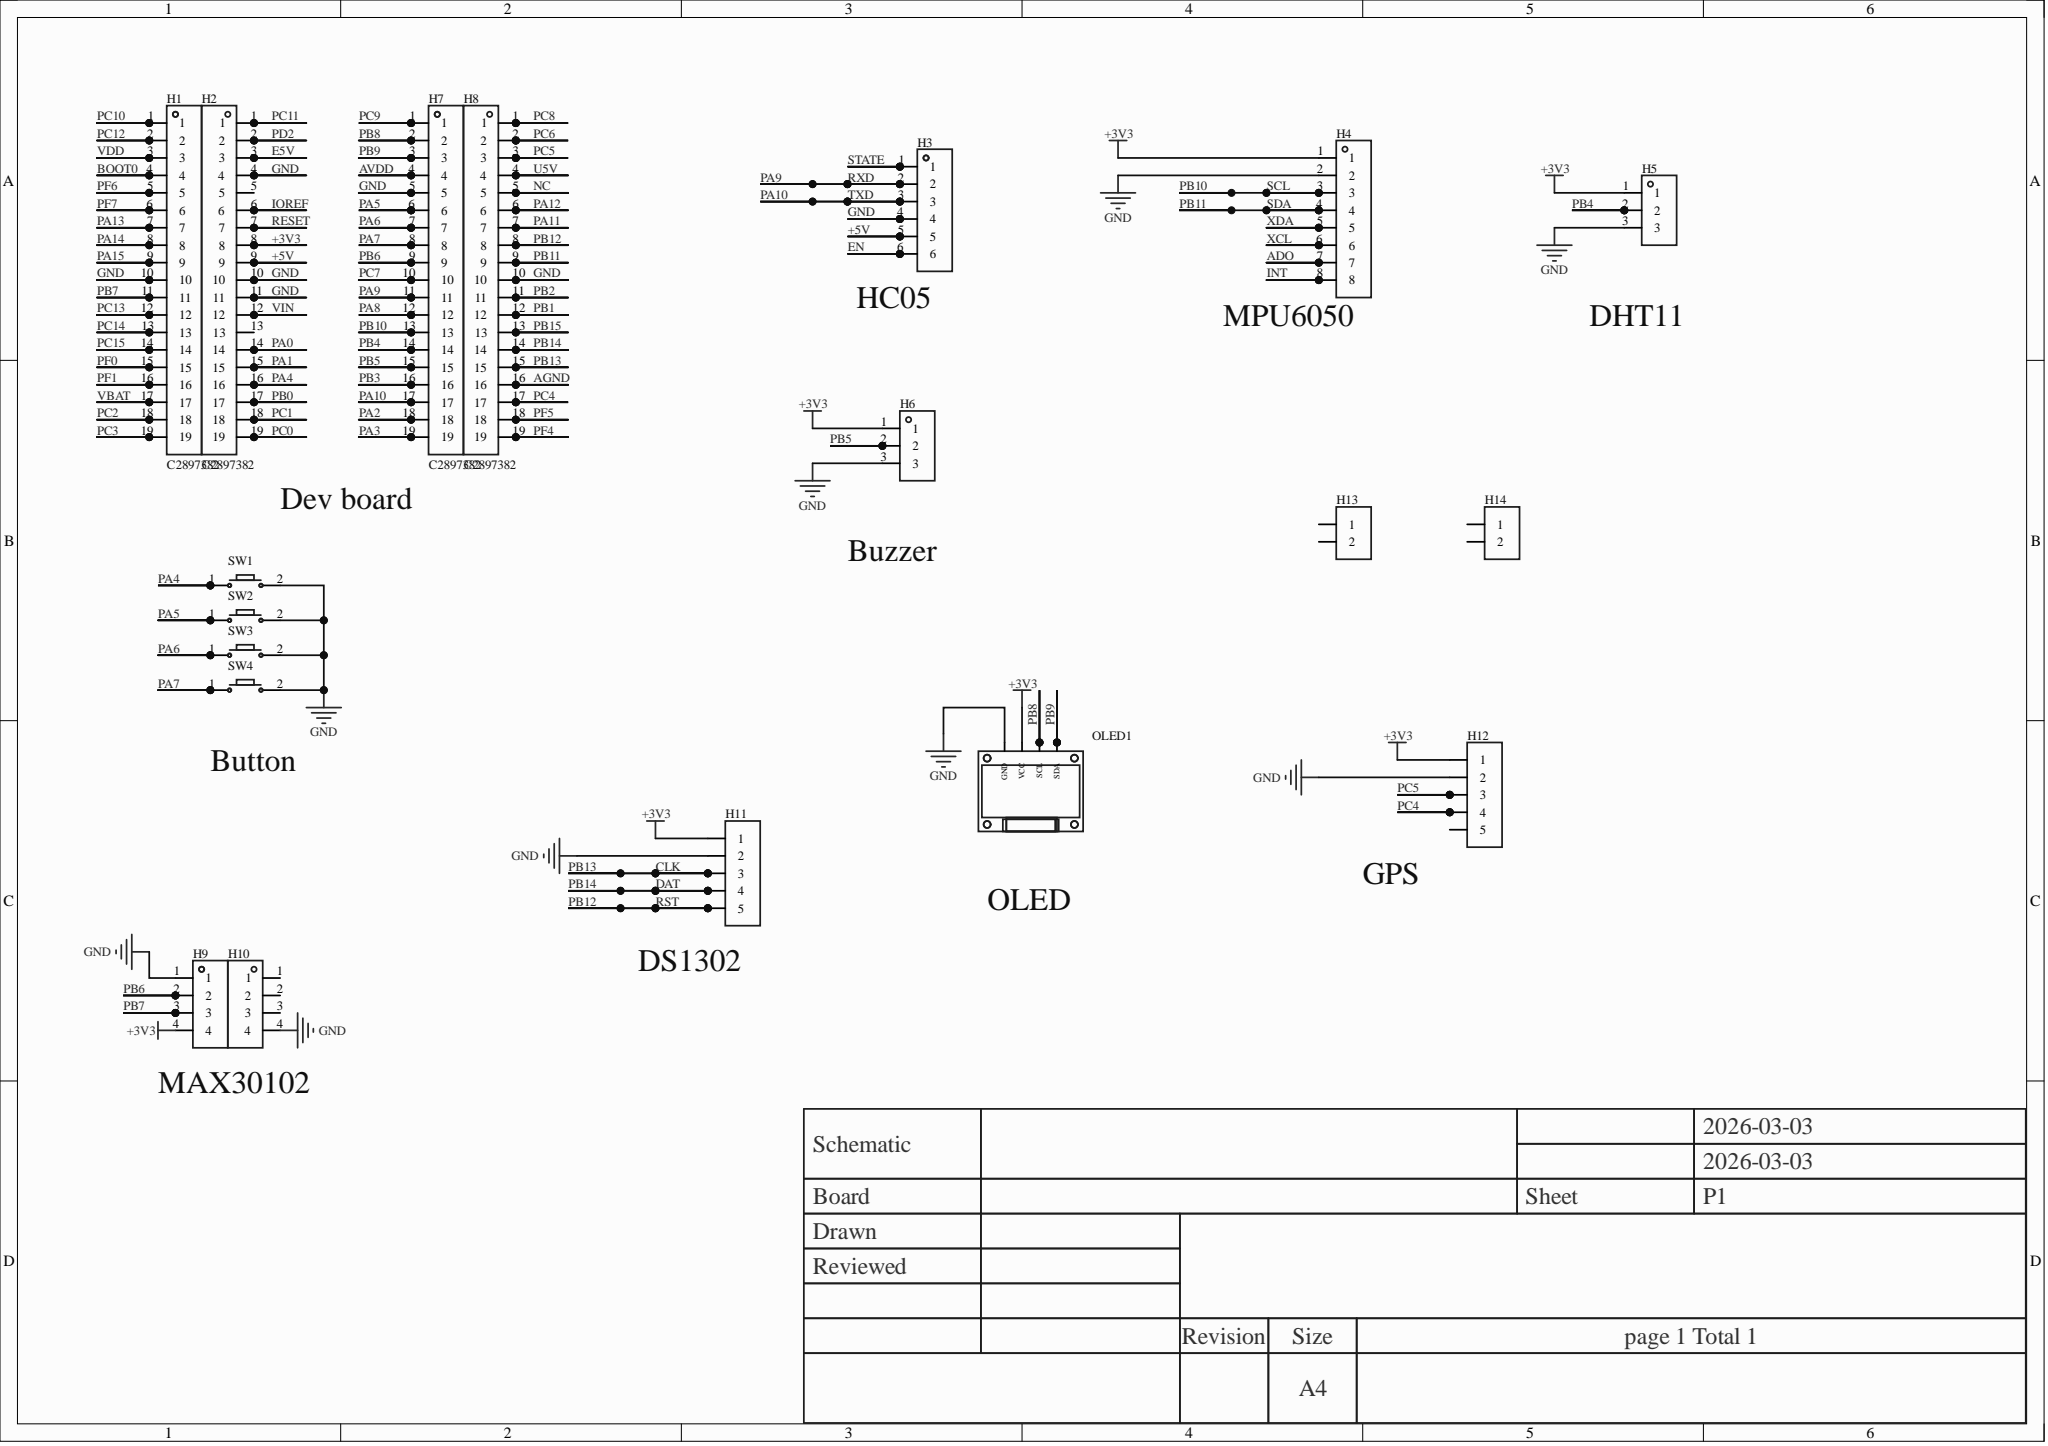Circuit board | Altium Designer | 19 parts | 22 nets
Bill of materials:
Comment,Description,Designator,Footprint,LibRef,Quantity
"C2897382","","H1, H2, H7, H8","HDR-TH_19P-P2.54-V-F","HDR-F_2.54_1x19P","4"
"","","H3","HDR-TH_6P-P2.54-V-F","HDR-F_2.54_1x6P","1"
"","","H4","HDR-TH_8P-P2.54-V-F-1","HDR-F_2.54_1x8P","1"
"","","H5, H6","HDR-TH_3P-P2.54-V-F","HDR-F_2.54_1x3P","2"
"","","H9, H10","HDR-TH_4P-P2.54-V-F","HDR-F_2.54_1x4P","2"
"","","H11, H12","HDR-TH_5P-P2.54-V-F","HDR-F_2.54_1x5P","2"
"","","H13, H14","HDR-TH_2P-P2.54-V-F","HDR-F_2.54_1x2P","2"
"","","OLED1","0.96OLED_4P","0.96OLED模块_4P","1"
"","","SW1, SW2, SW3, SW4","Key_SMD_3.6x6.1x2.5","Key_SMD_3.6x6.1x2.5","4"
Netlist (Protel format):
[
H1
HDR-TH_19P-P2.54-V-F
C2897382



]
[
H2
HDR-TH_19P-P2.54-V-F
C2897382



]
[
H3
HDR-TH_6P-P2.54-V-F




]
[
H4
HDR-TH_8P-P2.54-V-F-1




]
[
H5
HDR-TH_3P-P2.54-V-F




]
[
H6
HDR-TH_3P-P2.54-V-F




]
[
H7
HDR-TH_19P-P2.54-V-F
C2897382



]
[
H8
HDR-TH_19P-P2.54-V-F
C2897382



]
[
H9
HDR-TH_4P-P2.54-V-F




]
[
H10
HDR-TH_4P-P2.54-V-F




]
[
H11
HDR-TH_5P-P2.54-V-F




]
[
H12
HDR-TH_5P-P2.54-V-F




]
[
H13
HDR-TH_2P-P2.54-V-F




]
[
H14
HDR-TH_2P-P2.54-V-F




]
[
OLED1
0.96OLED_4P




]
[
SW1
Key_SMD_3.6x6.1x2.5




]
[
SW2
Key_SMD_3.6x6.1x2.5




]
[
SW3
Key_SMD_3.6x6.1x2.5




]
[
SW4
Key_SMD_3.6x6.1x2.5




]
(
PC5
H8-3
H12-3
)
(
PC4
H8-17
H12-4
)
(
PB12
H8-8
H11-5
)
(
PB11
H4-4
H8-9
)
(
PB10
H4-3
H7-13
)
(
PB9
H7-3
OLED1-4
)
(
PB8
H7-2
OLED1-3
)
(
PB7
H1-11
H9-3
)
(
PB6
H7-9
H9-2
)
(
PB5
H6-2
H7-15
)
(
PB4
H5-2
H7-14
)
(
PA10
H3-3
H7-17
)
(
PA9
H3-2
H7-11
)
(
PA7
H7-8
SW4-1
)
(
PA6
H7-7
SW3-1
)
(
PA5
H7-6
SW2-1
)
(
PA4
H2-16
SW1-1
)
(
GND
H1-10
H2-4
H2-10
H2-11
H3-4
H4-2
H5-3
H6-3
H7-5
H8-10
H9-1
H10-4
H11-2
H12-2
OLED1-1
SW1-2
SW2-2
SW3-2
SW4-2
)
(
DAT
H8-14
H11-4
)
(
CLK
H8-15
H11-3
)
(
+5V
H2-9
H3-5
)
(
+3V3
H2-8
H4-1
H5-1
H6-1
H9-4
H11-1
H12-1
OLED1-2
)